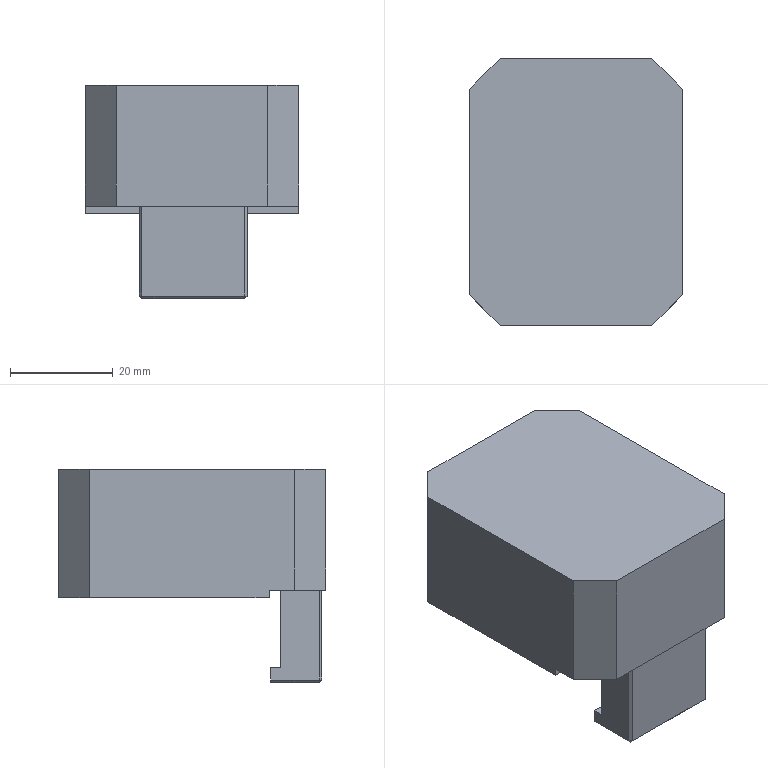Part | SolidWorks | features BaseBody 1 | 1 solid | 26 faces | box 41.5 x 52 x 41.5 mm | volume 54660 mm3 | plane 26
STEP:
#1=CARTESIAN_POINT('',(11.578,-12.01,25.));
#2=VERTEX_POINT('',#1);
#3=CARTESIAN_POINT('',(11.578,27.99,25.));
#4=VERTEX_POINT('',#3);
#5=CARTESIAN_POINT('',(11.578,7.99,25.));
#6=DIRECTION('',(0.,1.,0.));
#7=VECTOR('',#6,1000.);
#8=LINE('',#5,#7);
#9=EDGE_CURVE('',#2,#4,#8,.T.);
#10=ORIENTED_EDGE('',*,*,#9,.T.);
#11=CARTESIAN_POINT('',(5.578,33.99,25.));
#12=VERTEX_POINT('',#11);
#13=CARTESIAN_POINT('',(11.578,27.99,25.));
#14=DIRECTION('',(-0.7071,0.7071,0.));
#15=VECTOR('',#14,1000.);
#16=LINE('',#13,#15);
#17=EDGE_CURVE('',#4,#12,#16,.T.);
#18=ORIENTED_EDGE('',*,*,#17,.T.);
#19=CARTESIAN_POINT('',(-23.922,33.99,25.));
#20=VERTEX_POINT('',#19);
#21=CARTESIAN_POINT('',(-9.172,33.99,25.));
#22=DIRECTION('',(-1.,0.,0.));
#23=VECTOR('',#22,1000.);
#24=LINE('',#21,#23);
#25=EDGE_CURVE('',#12,#20,#24,.T.);
#26=ORIENTED_EDGE('',*,*,#25,.T.);
#27=CARTESIAN_POINT('',(-29.922,27.99,25.));
#28=VERTEX_POINT('',#27);
#29=CARTESIAN_POINT('',(-23.922,33.99,25.));
#30=DIRECTION('',(-0.7071,-0.7071,0.));
#31=VECTOR('',#30,1000.);
#32=LINE('',#29,#31);
#33=EDGE_CURVE('',#20,#28,#32,.T.);
#34=ORIENTED_EDGE('',*,*,#33,.T.);
#35=CARTESIAN_POINT('',(-29.922,-12.01,25.));
#36=VERTEX_POINT('',#35);
#37=CARTESIAN_POINT('',(-29.922,7.99,25.));
#38=DIRECTION('',(0.,-1.,0.));
#39=VECTOR('',#38,1000.);
#40=LINE('',#37,#39);
#41=EDGE_CURVE('',#28,#36,#40,.T.);
#42=ORIENTED_EDGE('',*,*,#41,.T.);
#43=CARTESIAN_POINT('',(-23.922,-18.01,25.));
#44=VERTEX_POINT('',#43);
#45=CARTESIAN_POINT('',(-29.922,-12.01,25.));
#46=DIRECTION('',(0.7071,-0.7071,0.));
#47=VECTOR('',#46,1000.);
#48=LINE('',#45,#47);
#49=EDGE_CURVE('',#36,#44,#48,.T.);
#50=ORIENTED_EDGE('',*,*,#49,.T.);
#51=CARTESIAN_POINT('',(5.578,-18.01,25.));
#52=VERTEX_POINT('',#51);
#53=CARTESIAN_POINT('',(-9.172,-18.01,25.));
#54=DIRECTION('',(1.,0.,0.));
#55=VECTOR('',#54,1000.);
#56=LINE('',#53,#55);
#57=EDGE_CURVE('',#44,#52,#56,.T.);
#58=ORIENTED_EDGE('',*,*,#57,.T.);
#59=CARTESIAN_POINT('',(5.578,-18.01,25.));
#60=DIRECTION('',(0.7071,0.7071,0.));
#61=VECTOR('',#60,1000.);
#62=LINE('',#59,#61);
#63=EDGE_CURVE('',#52,#2,#62,.T.);
#64=ORIENTED_EDGE('',*,*,#63,.T.);
#65=EDGE_LOOP('',(#10,#18,#26,#34,#42,#50,#58,#64));
#66=FACE_OUTER_BOUND('',#65,.T.);
#67=CARTESIAN_POINT('',(-9.172,7.99,25.));
#68=DIRECTION('',(0.,0.,1.));
#69=DIRECTION('',(1.,0.,0.));
#70=AXIS2_PLACEMENT_3D('',#67,#68,#69);
#71=PLANE('',#70);
#72=ADVANCED_FACE('',(#66),#71,.T.);
#73=CARTESIAN_POINT('',(11.578,27.99,0.));
#74=VERTEX_POINT('',#73);
#75=CARTESIAN_POINT('',(5.578,33.99,0.));
#76=VERTEX_POINT('',#75);
#77=CARTESIAN_POINT('',(5.578,33.99,0.));
#78=DIRECTION('',(-0.7071,0.7071,0.));
#79=VECTOR('',#78,1000.);
#80=LINE('',#77,#79);
#81=EDGE_CURVE('',#74,#76,#80,.T.);
#82=ORIENTED_EDGE('',*,*,#81,.T.);
#83=CARTESIAN_POINT('',(5.578,33.99,0.));
#84=DIRECTION('',(0.,0.,1.));
#85=VECTOR('',#84,1000.);
#86=LINE('',#83,#85);
#87=EDGE_CURVE('',#76,#12,#86,.T.);
#88=ORIENTED_EDGE('',*,*,#87,.T.);
#89=ORIENTED_EDGE('',*,*,#17,.F.);
#90=CARTESIAN_POINT('',(11.578,27.99,0.));
#91=DIRECTION('',(0.,0.,-1.));
#92=VECTOR('',#91,1000.);
#93=LINE('',#90,#92);
#94=EDGE_CURVE('',#4,#74,#93,.T.);
#95=ORIENTED_EDGE('',*,*,#94,.T.);
#96=EDGE_LOOP('',(#82,#88,#89,#95));
#97=FACE_OUTER_BOUND('',#96,.T.);
#98=CARTESIAN_POINT('',(5.578,33.99,0.));
#99=DIRECTION('',(0.7071,0.7071,0.));
#100=DIRECTION('',(-0.7071,0.7071,0.));
#101=AXIS2_PLACEMENT_3D('',#98,#99,#100);
#102=PLANE('',#101);
#103=ADVANCED_FACE('',(#97),#102,.T.);
#104=CARTESIAN_POINT('',(11.578,-12.01,1.5));
#105=VERTEX_POINT('',#104);
#106=CARTESIAN_POINT('',(11.578,-12.01,0.));
#107=DIRECTION('',(0.,0.,-1.));
#108=VECTOR('',#107,1000.);
#109=LINE('',#106,#108);
#110=EDGE_CURVE('',#2,#105,#109,.T.);
#111=ORIENTED_EDGE('',*,*,#110,.T.);
#112=CARTESIAN_POINT('',(11.578,-7.01,1.5));
#113=VERTEX_POINT('',#112);
#114=CARTESIAN_POINT('',(11.578,27.99,1.5));
#115=DIRECTION('',(0.,1.,0.));
#116=VECTOR('',#115,1000.);
#117=LINE('',#114,#116);
#118=EDGE_CURVE('',#105,#113,#117,.T.);
#119=ORIENTED_EDGE('',*,*,#118,.T.);
#120=CARTESIAN_POINT('',(11.578,-7.01,0.));
#121=VERTEX_POINT('',#120);
#122=CARTESIAN_POINT('',(11.578,-7.01,0.));
#123=DIRECTION('',(0.,0.,-1.));
#124=VECTOR('',#123,1000.);
#125=LINE('',#122,#124);
#126=EDGE_CURVE('',#113,#121,#125,.T.);
#127=ORIENTED_EDGE('',*,*,#126,.T.);
#128=CARTESIAN_POINT('',(11.578,27.99,0.));
#129=DIRECTION('',(0.,1.,0.));
#130=VECTOR('',#129,1000.);
#131=LINE('',#128,#130);
#132=EDGE_CURVE('',#121,#74,#131,.T.);
#133=ORIENTED_EDGE('',*,*,#132,.T.);
#134=ORIENTED_EDGE('',*,*,#94,.F.);
#135=ORIENTED_EDGE('',*,*,#9,.F.);
#136=EDGE_LOOP('',(#111,#119,#127,#133,#134,#135));
#137=FACE_OUTER_BOUND('',#136,.T.);
#138=CARTESIAN_POINT('',(11.578,27.99,0.));
#139=DIRECTION('',(1.,0.,0.));
#140=DIRECTION('',(0.,0.,-1.));
#141=AXIS2_PLACEMENT_3D('',#138,#139,#140);
#142=PLANE('',#141);
#143=ADVANCED_FACE('',(#137),#142,.T.);
#144=ORIENTED_EDGE('',*,*,#63,.F.);
#145=CARTESIAN_POINT('',(5.578,-18.01,1.5));
#146=VERTEX_POINT('',#145);
#147=CARTESIAN_POINT('',(5.578,-18.01,0.));
#148=DIRECTION('',(0.,0.,-1.));
#149=VECTOR('',#148,1000.);
#150=LINE('',#147,#149);
#151=EDGE_CURVE('',#52,#146,#150,.T.);
#152=ORIENTED_EDGE('',*,*,#151,.T.);
#153=CARTESIAN_POINT('',(11.578,-12.01,1.5));
#154=DIRECTION('',(0.7071,0.7071,0.));
#155=VECTOR('',#154,1000.);
#156=LINE('',#153,#155);
#157=EDGE_CURVE('',#146,#105,#156,.T.);
#158=ORIENTED_EDGE('',*,*,#157,.T.);
#159=ORIENTED_EDGE('',*,*,#110,.F.);
#160=EDGE_LOOP('',(#144,#152,#158,#159));
#161=FACE_OUTER_BOUND('',#160,.T.);
#162=CARTESIAN_POINT('',(11.578,-12.01,0.));
#163=DIRECTION('',(0.7071,-0.7071,0.));
#164=DIRECTION('',(0.7071,0.7071,0.));
#165=AXIS2_PLACEMENT_3D('',#162,#163,#164);
#166=PLANE('',#165);
#167=ADVANCED_FACE('',(#161),#166,.T.);
#168=ORIENTED_EDGE('',*,*,#57,.F.);
#169=CARTESIAN_POINT('',(-23.922,-18.01,1.5));
#170=VERTEX_POINT('',#169);
#171=CARTESIAN_POINT('',(-23.922,-18.01,0.));
#172=DIRECTION('',(0.,0.,-1.));
#173=VECTOR('',#172,1000.);
#174=LINE('',#171,#173);
#175=EDGE_CURVE('',#44,#170,#174,.T.);
#176=ORIENTED_EDGE('',*,*,#175,.T.);
#177=CARTESIAN_POINT('',(5.578,-18.01,1.5));
#178=DIRECTION('',(1.,0.,0.));
#179=VECTOR('',#178,1000.);
#180=LINE('',#177,#179);
#181=EDGE_CURVE('',#170,#146,#180,.T.);
#182=ORIENTED_EDGE('',*,*,#181,.T.);
#183=ORIENTED_EDGE('',*,*,#151,.F.);
#184=EDGE_LOOP('',(#168,#176,#182,#183));
#185=FACE_OUTER_BOUND('',#184,.T.);
#186=CARTESIAN_POINT('',(5.578,-18.01,0.));
#187=DIRECTION('',(0.,-1.,0.));
#188=DIRECTION('',(0.,0.,-1.));
#189=AXIS2_PLACEMENT_3D('',#186,#187,#188);
#190=PLANE('',#189);
#191=ADVANCED_FACE('',(#185),#190,.T.);
#192=ORIENTED_EDGE('',*,*,#49,.F.);
#193=CARTESIAN_POINT('',(-29.922,-12.01,1.5));
#194=VERTEX_POINT('',#193);
#195=CARTESIAN_POINT('',(-29.922,-12.01,0.));
#196=DIRECTION('',(0.,0.,-1.));
#197=VECTOR('',#196,1000.);
#198=LINE('',#195,#197);
#199=EDGE_CURVE('',#36,#194,#198,.T.);
#200=ORIENTED_EDGE('',*,*,#199,.T.);
#201=CARTESIAN_POINT('',(-23.922,-18.01,1.5));
#202=DIRECTION('',(0.7071,-0.7071,0.));
#203=VECTOR('',#202,1000.);
#204=LINE('',#201,#203);
#205=EDGE_CURVE('',#194,#170,#204,.T.);
#206=ORIENTED_EDGE('',*,*,#205,.T.);
#207=ORIENTED_EDGE('',*,*,#175,.F.);
#208=EDGE_LOOP('',(#192,#200,#206,#207));
#209=FACE_OUTER_BOUND('',#208,.T.);
#210=CARTESIAN_POINT('',(-23.922,-18.01,0.));
#211=DIRECTION('',(-0.7071,-0.7071,0.));
#212=DIRECTION('',(0.7071,-0.7071,0.));
#213=AXIS2_PLACEMENT_3D('',#210,#211,#212);
#214=PLANE('',#213);
#215=ADVANCED_FACE('',(#209),#214,.T.);
#216=CARTESIAN_POINT('',(-29.922,27.99,0.));
#217=VERTEX_POINT('',#216);
#218=CARTESIAN_POINT('',(-29.922,-7.01,0.));
#219=VERTEX_POINT('',#218);
#220=CARTESIAN_POINT('',(-29.922,-12.01,0.));
#221=DIRECTION('',(0.,-1.,0.));
#222=VECTOR('',#221,1000.);
#223=LINE('',#220,#222);
#224=EDGE_CURVE('',#217,#219,#223,.T.);
#225=ORIENTED_EDGE('',*,*,#224,.T.);
#226=CARTESIAN_POINT('',(-29.922,-7.01,1.5));
#227=VERTEX_POINT('',#226);
#228=CARTESIAN_POINT('',(-29.922,-7.01,0.));
#229=DIRECTION('',(0.,0.,1.));
#230=VECTOR('',#229,1000.);
#231=LINE('',#228,#230);
#232=EDGE_CURVE('',#219,#227,#231,.T.);
#233=ORIENTED_EDGE('',*,*,#232,.T.);
#234=CARTESIAN_POINT('',(-29.922,-12.01,1.5));
#235=DIRECTION('',(0.,-1.,0.));
#236=VECTOR('',#235,1000.);
#237=LINE('',#234,#236);
#238=EDGE_CURVE('',#227,#194,#237,.T.);
#239=ORIENTED_EDGE('',*,*,#238,.T.);
#240=ORIENTED_EDGE('',*,*,#199,.F.);
#241=ORIENTED_EDGE('',*,*,#41,.F.);
#242=CARTESIAN_POINT('',(-29.922,27.99,0.));
#243=DIRECTION('',(0.,0.,-1.));
#244=VECTOR('',#243,1000.);
#245=LINE('',#242,#244);
#246=EDGE_CURVE('',#28,#217,#245,.T.);
#247=ORIENTED_EDGE('',*,*,#246,.T.);
#248=EDGE_LOOP('',(#225,#233,#239,#240,#241,#247));
#249=FACE_OUTER_BOUND('',#248,.T.);
#250=CARTESIAN_POINT('',(-29.922,-12.01,0.));
#251=DIRECTION('',(-1.,0.,0.));
#252=DIRECTION('',(0.,0.,1.));
#253=AXIS2_PLACEMENT_3D('',#250,#251,#252);
#254=PLANE('',#253);
#255=ADVANCED_FACE('',(#249),#254,.T.);
#256=CARTESIAN_POINT('',(-23.922,33.99,0.));
#257=VERTEX_POINT('',#256);
#258=CARTESIAN_POINT('',(-29.922,27.99,0.));
#259=DIRECTION('',(-0.7071,-0.7071,0.));
#260=VECTOR('',#259,1000.);
#261=LINE('',#258,#260);
#262=EDGE_CURVE('',#257,#217,#261,.T.);
#263=ORIENTED_EDGE('',*,*,#262,.T.);
#264=ORIENTED_EDGE('',*,*,#246,.F.);
#265=ORIENTED_EDGE('',*,*,#33,.F.);
#266=CARTESIAN_POINT('',(-23.922,33.99,0.));
#267=DIRECTION('',(0.,0.,-1.));
#268=VECTOR('',#267,1000.);
#269=LINE('',#266,#268);
#270=EDGE_CURVE('',#20,#257,#269,.T.);
#271=ORIENTED_EDGE('',*,*,#270,.T.);
#272=EDGE_LOOP('',(#263,#264,#265,#271));
#273=FACE_OUTER_BOUND('',#272,.T.);
#274=CARTESIAN_POINT('',(-29.922,27.99,0.));
#275=DIRECTION('',(-0.7071,0.7071,0.));
#276=DIRECTION('',(-0.7071,-0.7071,0.));
#277=AXIS2_PLACEMENT_3D('',#274,#275,#276);
#278=PLANE('',#277);
#279=ADVANCED_FACE('',(#273),#278,.T.);
#280=CARTESIAN_POINT('',(-23.922,33.99,0.));
#281=DIRECTION('',(-1.,0.,0.));
#282=VECTOR('',#281,1000.);
#283=LINE('',#280,#282);
#284=EDGE_CURVE('',#76,#257,#283,.T.);
#285=ORIENTED_EDGE('',*,*,#284,.T.);
#286=ORIENTED_EDGE('',*,*,#270,.F.);
#287=ORIENTED_EDGE('',*,*,#25,.F.);
#288=ORIENTED_EDGE('',*,*,#87,.F.);
#289=EDGE_LOOP('',(#285,#286,#287,#288));
#290=FACE_OUTER_BOUND('',#289,.T.);
#291=CARTESIAN_POINT('',(-23.922,33.99,0.));
#292=DIRECTION('',(0.,1.,0.));
#293=DIRECTION('',(0.,0.,1.));
#294=AXIS2_PLACEMENT_3D('',#291,#292,#293);
#295=PLANE('',#294);
#296=ADVANCED_FACE('',(#290),#295,.T.);
#297=ORIENTED_EDGE('',*,*,#224,.F.);
#298=ORIENTED_EDGE('',*,*,#262,.F.);
#299=ORIENTED_EDGE('',*,*,#284,.F.);
#300=ORIENTED_EDGE('',*,*,#81,.F.);
#301=ORIENTED_EDGE('',*,*,#132,.F.);
#302=CARTESIAN_POINT('',(-9.172,-7.01,0.));
#303=DIRECTION('',(1.,0.,0.));
#304=VECTOR('',#303,1000.);
#305=LINE('',#302,#304);
#306=EDGE_CURVE('',#219,#121,#305,.T.);
#307=ORIENTED_EDGE('',*,*,#306,.F.);
#308=EDGE_LOOP('',(#297,#298,#299,#300,#301,#307));
#309=FACE_OUTER_BOUND('',#308,.T.);
#310=CARTESIAN_POINT('',(-9.172,7.99,0.));
#311=DIRECTION('',(0.,0.,1.));
#312=DIRECTION('',(1.,0.,0.));
#313=AXIS2_PLACEMENT_3D('',#310,#311,#312);
#314=PLANE('',#313);
#315=ADVANCED_FACE('',(#309),#314,.F.);
#316=CARTESIAN_POINT('',(-18.922,-17.31,1.5));
#317=VERTEX_POINT('',#316);
#318=CARTESIAN_POINT('',(-19.422,-16.81,1.5));
#319=VERTEX_POINT('',#318);
#320=CARTESIAN_POINT('',(-19.172,-17.06,1.5));
#321=DIRECTION('',(-0.7071,0.7071,0.));
#322=VECTOR('',#321,1000.);
#323=LINE('',#320,#322);
#324=EDGE_CURVE('',#317,#319,#323,.T.);
#325=ORIENTED_EDGE('',*,*,#324,.F.);
#326=CARTESIAN_POINT('',(1.078,-17.31,1.5));
#327=VERTEX_POINT('',#326);
#328=CARTESIAN_POINT('',(-9.172,-17.31,1.5));
#329=DIRECTION('',(-1.,0.,0.));
#330=VECTOR('',#329,1000.);
#331=LINE('',#328,#330);
#332=EDGE_CURVE('',#327,#317,#331,.T.);
#333=ORIENTED_EDGE('',*,*,#332,.F.);
#334=CARTESIAN_POINT('',(1.578,-16.81,1.5));
#335=VERTEX_POINT('',#334);
#336=CARTESIAN_POINT('',(1.328,-17.06,1.5));
#337=DIRECTION('',(-0.7071,-0.7071,0.));
#338=VECTOR('',#337,1000.);
#339=LINE('',#336,#338);
#340=EDGE_CURVE('',#335,#327,#339,.T.);
#341=ORIENTED_EDGE('',*,*,#340,.F.);
#342=CARTESIAN_POINT('',(1.578,-9.31,1.5));
#343=VERTEX_POINT('',#342);
#344=CARTESIAN_POINT('',(1.578,-11.963,1.5));
#345=DIRECTION('',(0.,-1.,0.));
#346=VECTOR('',#345,1000.);
#347=LINE('',#344,#346);
#348=EDGE_CURVE('',#343,#335,#347,.T.);
#349=ORIENTED_EDGE('',*,*,#348,.F.);
#350=CARTESIAN_POINT('',(-19.422,-9.31,1.5));
#351=VERTEX_POINT('',#350);
#352=CARTESIAN_POINT('',(-9.172,-9.31,1.5));
#353=DIRECTION('',(1.,0.,0.));
#354=VECTOR('',#353,1000.);
#355=LINE('',#352,#354);
#356=EDGE_CURVE('',#351,#343,#355,.T.);
#357=ORIENTED_EDGE('',*,*,#356,.F.);
#358=CARTESIAN_POINT('',(-19.422,-11.963,1.5));
#359=DIRECTION('',(0.,1.,0.));
#360=VECTOR('',#359,1000.);
#361=LINE('',#358,#360);
#362=EDGE_CURVE('',#319,#351,#361,.T.);
#363=ORIENTED_EDGE('',*,*,#362,.F.);
#364=EDGE_LOOP('',(#325,#333,#341,#349,#357,#363));
#365=FACE_BOUND('',#364,.T.);
#366=ORIENTED_EDGE('',*,*,#205,.F.);
#367=ORIENTED_EDGE('',*,*,#238,.F.);
#368=CARTESIAN_POINT('',(-9.172,-7.01,1.5));
#369=DIRECTION('',(-1.,0.,0.));
#370=VECTOR('',#369,1000.);
#371=LINE('',#368,#370);
#372=EDGE_CURVE('',#113,#227,#371,.T.);
#373=ORIENTED_EDGE('',*,*,#372,.F.);
#374=ORIENTED_EDGE('',*,*,#118,.F.);
#375=ORIENTED_EDGE('',*,*,#157,.F.);
#376=ORIENTED_EDGE('',*,*,#181,.F.);
#377=EDGE_LOOP('',(#366,#367,#373,#374,#375,#376));
#378=FACE_OUTER_BOUND('',#377,.T.);
#379=CARTESIAN_POINT('',(-9.172,-11.963,1.5));
#380=DIRECTION('',(0.,0.,1.));
#381=DIRECTION('',(1.,0.,0.));
#382=AXIS2_PLACEMENT_3D('',#379,#380,#381);
#383=PLANE('',#382);
#384=ADVANCED_FACE('',(#365,#378),#383,.F.);
#385=ORIENTED_EDGE('',*,*,#232,.F.);
#386=ORIENTED_EDGE('',*,*,#306,.T.);
#387=ORIENTED_EDGE('',*,*,#126,.F.);
#388=ORIENTED_EDGE('',*,*,#372,.T.);
#389=EDGE_LOOP('',(#385,#386,#387,#388));
#390=FACE_OUTER_BOUND('',#389,.T.);
#391=CARTESIAN_POINT('',(-29.922,-7.01,0.));
#392=DIRECTION('',(0.,1.,0.));
#393=DIRECTION('',(0.,0.,1.));
#394=AXIS2_PLACEMENT_3D('',#391,#392,#393);
#395=PLANE('',#394);
#396=ADVANCED_FACE('',(#390),#395,.F.);
#397=CARTESIAN_POINT('',(-19.422,-7.31,-13.5));
#398=VERTEX_POINT('',#397);
#399=CARTESIAN_POINT('',(-19.422,-7.31,-16.));
#400=VERTEX_POINT('',#399);
#401=CARTESIAN_POINT('',(-19.422,-7.31,1.5));
#402=DIRECTION('',(0.,0.,-1.));
#403=VECTOR('',#402,1000.);
#404=LINE('',#401,#403);
#405=EDGE_CURVE('',#398,#400,#404,.T.);
#406=ORIENTED_EDGE('',*,*,#405,.T.);
#407=CARTESIAN_POINT('',(-19.422,-16.81,-16.));
#408=VERTEX_POINT('',#407);
#409=CARTESIAN_POINT('',(-19.422,-9.31,-16.));
#410=DIRECTION('',(0.,-1.,0.));
#411=VECTOR('',#410,1000.);
#412=LINE('',#409,#411);
#413=EDGE_CURVE('',#400,#408,#412,.T.);
#414=ORIENTED_EDGE('',*,*,#413,.T.);
#415=CARTESIAN_POINT('',(-19.422,-16.81,1.5));
#416=DIRECTION('',(0.,0.,1.));
#417=VECTOR('',#416,1000.);
#418=LINE('',#415,#417);
#419=EDGE_CURVE('',#408,#319,#418,.T.);
#420=ORIENTED_EDGE('',*,*,#419,.T.);
#421=ORIENTED_EDGE('',*,*,#362,.T.);
#422=CARTESIAN_POINT('',(-19.422,-9.31,-13.5));
#423=VERTEX_POINT('',#422);
#424=CARTESIAN_POINT('',(-19.422,-9.31,1.5));
#425=DIRECTION('',(0.,0.,-1.));
#426=VECTOR('',#425,1000.);
#427=LINE('',#424,#426);
#428=EDGE_CURVE('',#351,#423,#427,.T.);
#429=ORIENTED_EDGE('',*,*,#428,.T.);
#430=CARTESIAN_POINT('',(-19.422,-9.31,-13.5));
#431=DIRECTION('',(0.,1.,0.));
#432=VECTOR('',#431,1000.);
#433=LINE('',#430,#432);
#434=EDGE_CURVE('',#423,#398,#433,.T.);
#435=ORIENTED_EDGE('',*,*,#434,.T.);
#436=EDGE_LOOP('',(#406,#414,#420,#421,#429,#435));
#437=FACE_OUTER_BOUND('',#436,.T.);
#438=CARTESIAN_POINT('',(-19.422,-9.31,1.5));
#439=DIRECTION('',(-1.,0.,0.));
#440=DIRECTION('',(0.,0.,1.));
#441=AXIS2_PLACEMENT_3D('',#438,#439,#440);
#442=PLANE('',#441);
#443=ADVANCED_FACE('',(#437),#442,.T.);
#444=CARTESIAN_POINT('',(1.078,-17.31,-16.));
#445=VERTEX_POINT('',#444);
#446=CARTESIAN_POINT('',(1.078,-17.31,1.5));
#447=DIRECTION('',(0.,0.,1.));
#448=VECTOR('',#447,1000.);
#449=LINE('',#446,#448);
#450=EDGE_CURVE('',#445,#327,#449,.T.);
#451=ORIENTED_EDGE('',*,*,#450,.T.);
#452=ORIENTED_EDGE('',*,*,#332,.T.);
#453=CARTESIAN_POINT('',(-18.922,-17.31,-16.));
#454=VERTEX_POINT('',#453);
#455=CARTESIAN_POINT('',(-18.922,-17.31,1.5));
#456=DIRECTION('',(0.,0.,-1.));
#457=VECTOR('',#456,1000.);
#458=LINE('',#455,#457);
#459=EDGE_CURVE('',#317,#454,#458,.T.);
#460=ORIENTED_EDGE('',*,*,#459,.T.);
#461=CARTESIAN_POINT('',(-19.422,-17.31,-16.));
#462=DIRECTION('',(1.,0.,0.));
#463=VECTOR('',#462,1000.);
#464=LINE('',#461,#463);
#465=EDGE_CURVE('',#454,#445,#464,.T.);
#466=ORIENTED_EDGE('',*,*,#465,.T.);
#467=EDGE_LOOP('',(#451,#452,#460,#466));
#468=FACE_OUTER_BOUND('',#467,.T.);
#469=CARTESIAN_POINT('',(-19.422,-17.31,1.5));
#470=DIRECTION('',(0.,-1.,0.));
#471=DIRECTION('',(0.,0.,-1.));
#472=AXIS2_PLACEMENT_3D('',#469,#470,#471);
#473=PLANE('',#472);
#474=ADVANCED_FACE('',(#468),#473,.T.);
#475=CARTESIAN_POINT('',(1.578,-9.31,-13.5));
#476=VERTEX_POINT('',#475);
#477=CARTESIAN_POINT('',(1.578,-9.31,1.5));
#478=DIRECTION('',(0.,0.,1.));
#479=VECTOR('',#478,1000.);
#480=LINE('',#477,#479);
#481=EDGE_CURVE('',#476,#343,#480,.T.);
#482=ORIENTED_EDGE('',*,*,#481,.T.);
#483=ORIENTED_EDGE('',*,*,#348,.T.);
#484=CARTESIAN_POINT('',(1.578,-16.81,-16.));
#485=VERTEX_POINT('',#484);
#486=CARTESIAN_POINT('',(1.578,-16.81,1.5));
#487=DIRECTION('',(0.,0.,-1.));
#488=VECTOR('',#487,1000.);
#489=LINE('',#486,#488);
#490=EDGE_CURVE('',#335,#485,#489,.T.);
#491=ORIENTED_EDGE('',*,*,#490,.T.);
#492=CARTESIAN_POINT('',(1.578,-7.31,-16.));
#493=VERTEX_POINT('',#492);
#494=CARTESIAN_POINT('',(1.578,-17.31,-16.));
#495=DIRECTION('',(0.,1.,0.));
#496=VECTOR('',#495,1000.);
#497=LINE('',#494,#496);
#498=EDGE_CURVE('',#485,#493,#497,.T.);
#499=ORIENTED_EDGE('',*,*,#498,.T.);
#500=CARTESIAN_POINT('',(1.578,-7.31,-13.5));
#501=VERTEX_POINT('',#500);
#502=CARTESIAN_POINT('',(1.578,-7.31,1.5));
#503=DIRECTION('',(0.,0.,1.));
#504=VECTOR('',#503,1000.);
#505=LINE('',#502,#504);
#506=EDGE_CURVE('',#493,#501,#505,.T.);
#507=ORIENTED_EDGE('',*,*,#506,.T.);
#508=CARTESIAN_POINT('',(1.578,-17.31,-13.5));
#509=DIRECTION('',(0.,-1.,0.));
#510=VECTOR('',#509,1000.);
#511=LINE('',#508,#510);
#512=EDGE_CURVE('',#501,#476,#511,.T.);
#513=ORIENTED_EDGE('',*,*,#512,.T.);
#514=EDGE_LOOP('',(#482,#483,#491,#499,#507,#513));
#515=FACE_OUTER_BOUND('',#514,.T.);
#516=CARTESIAN_POINT('',(1.578,-17.31,1.5));
#517=DIRECTION('',(1.,0.,0.));
#518=DIRECTION('',(0.,0.,-1.));
#519=AXIS2_PLACEMENT_3D('',#516,#517,#518);
#520=PLANE('',#519);
#521=ADVANCED_FACE('',(#515),#520,.T.);
#522=ORIENTED_EDGE('',*,*,#356,.T.);
#523=ORIENTED_EDGE('',*,*,#481,.F.);
#524=CARTESIAN_POINT('',(1.578,-9.31,-13.5));
#525=DIRECTION('',(-1.,0.,0.));
#526=VECTOR('',#525,1000.);
#527=LINE('',#524,#526);
#528=EDGE_CURVE('',#476,#423,#527,.T.);
#529=ORIENTED_EDGE('',*,*,#528,.T.);
#530=ORIENTED_EDGE('',*,*,#428,.F.);
#531=EDGE_LOOP('',(#522,#523,#529,#530));
#532=FACE_OUTER_BOUND('',#531,.T.);
#533=CARTESIAN_POINT('',(1.578,-9.31,1.5));
#534=DIRECTION('',(0.,1.,0.));
#535=DIRECTION('',(0.,0.,1.));
#536=AXIS2_PLACEMENT_3D('',#533,#534,#535);
#537=PLANE('',#536);
#538=ADVANCED_FACE('',(#532),#537,.T.);
#539=ORIENTED_EDGE('',*,*,#413,.F.);
#540=CARTESIAN_POINT('',(-18.922,-7.31,-16.5));
#541=VERTEX_POINT('',#540);
#542=CARTESIAN_POINT('',(-19.172,-7.31,-16.25));
#543=DIRECTION('',(0.7071,0.,-0.7071));
#544=VECTOR('',#543,1000.);
#545=LINE('',#542,#544);
#546=EDGE_CURVE('',#400,#541,#545,.T.);
#547=ORIENTED_EDGE('',*,*,#546,.T.);
#548=CARTESIAN_POINT('',(-18.922,-16.81,-16.5));
#549=VERTEX_POINT('',#548);
#550=CARTESIAN_POINT('',(-18.922,-11.31,-16.5));
#551=DIRECTION('',(0.,-1.,0.));
#552=VECTOR('',#551,1000.);
#553=LINE('',#550,#552);
#554=EDGE_CURVE('',#541,#549,#553,.T.);
#555=ORIENTED_EDGE('',*,*,#554,.T.);
#556=CARTESIAN_POINT('',(-19.172,-16.81,-16.25));
#557=DIRECTION('',(-0.7071,0.,0.7071));
#558=VECTOR('',#557,1000.);
#559=LINE('',#556,#558);
#560=EDGE_CURVE('',#549,#408,#559,.T.);
#561=ORIENTED_EDGE('',*,*,#560,.T.);
#562=EDGE_LOOP('',(#539,#547,#555,#561));
#563=FACE_OUTER_BOUND('',#562,.T.);
#564=CARTESIAN_POINT('',(-19.172,-11.31,-16.25));
#565=DIRECTION('',(-0.7071,0.,-0.7071));
#566=DIRECTION('',(-0.7071,0.,0.7071));
#567=AXIS2_PLACEMENT_3D('',#564,#565,#566);
#568=PLANE('',#567);
#569=ADVANCED_FACE('',(#563),#568,.T.);
#570=ORIENTED_EDGE('',*,*,#506,.F.);
#571=CARTESIAN_POINT('',(1.078,-7.31,-16.5));
#572=VERTEX_POINT('',#571);
#573=CARTESIAN_POINT('',(1.578,-7.31,-16.));
#574=DIRECTION('',(-0.7071,0.,-0.7071));
#575=VECTOR('',#574,1000.);
#576=LINE('',#573,#575);
#577=EDGE_CURVE('',#493,#572,#576,.T.);
#578=ORIENTED_EDGE('',*,*,#577,.T.);
#579=CARTESIAN_POINT('',(-8.922,-7.31,-16.5));
#580=DIRECTION('',(-1.,0.,0.));
#581=VECTOR('',#580,1000.);
#582=LINE('',#579,#581);
#583=EDGE_CURVE('',#572,#541,#582,.T.);
#584=ORIENTED_EDGE('',*,*,#583,.T.);
#585=ORIENTED_EDGE('',*,*,#546,.F.);
#586=ORIENTED_EDGE('',*,*,#405,.F.);
#587=CARTESIAN_POINT('',(-8.922,-7.31,-13.5));
#588=DIRECTION('',(1.,0.,0.));
#589=VECTOR('',#588,1000.);
#590=LINE('',#587,#589);
#591=EDGE_CURVE('',#398,#501,#590,.T.);
#592=ORIENTED_EDGE('',*,*,#591,.T.);
#593=EDGE_LOOP('',(#570,#578,#584,#585,#586,#592));
#594=FACE_OUTER_BOUND('',#593,.T.);
#595=CARTESIAN_POINT('',(-8.922,-7.31,-14.979));
#596=DIRECTION('',(0.,1.,0.));
#597=DIRECTION('',(0.,0.,1.));
#598=AXIS2_PLACEMENT_3D('',#595,#596,#597);
#599=PLANE('',#598);
#600=ADVANCED_FACE('',(#594),#599,.T.);
#601=ORIENTED_EDGE('',*,*,#528,.F.);
#602=ORIENTED_EDGE('',*,*,#512,.F.);
#603=ORIENTED_EDGE('',*,*,#591,.F.);
#604=ORIENTED_EDGE('',*,*,#434,.F.);
#605=EDGE_LOOP('',(#601,#602,#603,#604));
#606=FACE_OUTER_BOUND('',#605,.T.);
#607=CARTESIAN_POINT('',(1.578,-9.31,-13.5));
#608=DIRECTION('',(0.,0.,1.));
#609=DIRECTION('',(1.,0.,0.));
#610=AXIS2_PLACEMENT_3D('',#607,#608,#609);
#611=PLANE('',#610);
#612=ADVANCED_FACE('',(#606),#611,.T.);
#613=CARTESIAN_POINT('',(-19.172,-17.06,-16.));
#614=DIRECTION('',(0.7071,-0.7071,0.));
#615=VECTOR('',#614,1000.);
#616=LINE('',#613,#615);
#617=EDGE_CURVE('',#408,#454,#616,.T.);
#618=ORIENTED_EDGE('',*,*,#617,.T.);
#619=ORIENTED_EDGE('',*,*,#459,.F.);
#620=ORIENTED_EDGE('',*,*,#324,.T.);
#621=ORIENTED_EDGE('',*,*,#419,.F.);
#622=EDGE_LOOP('',(#618,#619,#620,#621));
#623=FACE_OUTER_BOUND('',#622,.T.);
#624=CARTESIAN_POINT('',(-19.172,-17.06,1.5));
#625=DIRECTION('',(-0.7071,-0.7071,0.));
#626=DIRECTION('',(0.7071,-0.7071,0.));
#627=AXIS2_PLACEMENT_3D('',#624,#625,#626);
#628=PLANE('',#627);
#629=ADVANCED_FACE('',(#623),#628,.T.);
#630=CARTESIAN_POINT('',(1.328,-17.06,-16.));
#631=DIRECTION('',(0.7071,0.7071,0.));
#632=VECTOR('',#631,1000.);
#633=LINE('',#630,#632);
#634=EDGE_CURVE('',#445,#485,#633,.T.);
#635=ORIENTED_EDGE('',*,*,#634,.T.);
#636=ORIENTED_EDGE('',*,*,#490,.F.);
#637=ORIENTED_EDGE('',*,*,#340,.T.);
#638=ORIENTED_EDGE('',*,*,#450,.F.);
#639=EDGE_LOOP('',(#635,#636,#637,#638));
#640=FACE_OUTER_BOUND('',#639,.T.);
#641=CARTESIAN_POINT('',(1.328,-17.06,1.5));
#642=DIRECTION('',(0.7071,-0.7071,0.));
#643=DIRECTION('',(0.7071,0.7071,0.));
#644=AXIS2_PLACEMENT_3D('',#641,#642,#643);
#645=PLANE('',#644);
#646=ADVANCED_FACE('',(#640),#645,.T.);
#647=CARTESIAN_POINT('',(-18.922,-17.06,-16.25));
#648=DIRECTION('',(0.,0.7071,-0.7071));
#649=VECTOR('',#648,1000.);
#650=LINE('',#647,#649);
#651=EDGE_CURVE('',#454,#549,#650,.T.);
#652=ORIENTED_EDGE('',*,*,#651,.T.);
#653=CARTESIAN_POINT('',(1.078,-16.81,-16.5));
#654=VERTEX_POINT('',#653);
#655=CARTESIAN_POINT('',(-14.172,-16.81,-16.5));
#656=DIRECTION('',(1.,0.,0.));
#657=VECTOR('',#656,1000.);
#658=LINE('',#655,#657);
#659=EDGE_CURVE('',#549,#654,#658,.T.);
#660=ORIENTED_EDGE('',*,*,#659,.T.);
#661=CARTESIAN_POINT('',(1.078,-17.06,-16.25));
#662=DIRECTION('',(0.,-0.7071,0.7071));
#663=VECTOR('',#662,1000.);
#664=LINE('',#661,#663);
#665=EDGE_CURVE('',#654,#445,#664,.T.);
#666=ORIENTED_EDGE('',*,*,#665,.T.);
#667=ORIENTED_EDGE('',*,*,#465,.F.);
#668=EDGE_LOOP('',(#652,#660,#666,#667));
#669=FACE_OUTER_BOUND('',#668,.T.);
#670=CARTESIAN_POINT('',(-14.172,-17.06,-16.25));
#671=DIRECTION('',(0.,-0.7071,-0.7071));
#672=DIRECTION('',(0.,0.7071,-0.7071));
#673=AXIS2_PLACEMENT_3D('',#670,#671,#672);
#674=PLANE('',#673);
#675=ADVANCED_FACE('',(#669),#674,.T.);
#676=CARTESIAN_POINT('',(1.078,-15.31,-16.5));
#677=DIRECTION('',(0.,1.,0.));
#678=VECTOR('',#677,1000.);
#679=LINE('',#676,#678);
#680=EDGE_CURVE('',#654,#572,#679,.T.);
#681=ORIENTED_EDGE('',*,*,#680,.T.);
#682=ORIENTED_EDGE('',*,*,#577,.F.);
#683=ORIENTED_EDGE('',*,*,#498,.F.);
#684=CARTESIAN_POINT('',(1.328,-16.81,-16.25));
#685=DIRECTION('',(-0.7071,0.,-0.7071));
#686=VECTOR('',#685,1000.);
#687=LINE('',#684,#686);
#688=EDGE_CURVE('',#485,#654,#687,.T.);
#689=ORIENTED_EDGE('',*,*,#688,.T.);
#690=EDGE_LOOP('',(#681,#682,#683,#689));
#691=FACE_OUTER_BOUND('',#690,.T.);
#692=CARTESIAN_POINT('',(1.328,-15.31,-16.25));
#693=DIRECTION('',(0.7071,0.,-0.7071));
#694=DIRECTION('',(-0.7071,0.,-0.7071));
#695=AXIS2_PLACEMENT_3D('',#692,#693,#694);
#696=PLANE('',#695);
#697=ADVANCED_FACE('',(#691),#696,.T.);
#698=ORIENTED_EDGE('',*,*,#651,.F.);
#699=ORIENTED_EDGE('',*,*,#617,.F.);
#700=ORIENTED_EDGE('',*,*,#560,.F.);
#701=EDGE_LOOP('',(#698,#699,#700));
#702=FACE_OUTER_BOUND('',#701,.T.);
#703=CARTESIAN_POINT('',(-19.172,-17.06,-16.));
#704=DIRECTION('',(-0.5774,-0.5774,-0.5774));
#705=DIRECTION('',(0.,0.7071,-0.7071));
#706=AXIS2_PLACEMENT_3D('',#703,#704,#705);
#707=PLANE('',#706);
#708=ADVANCED_FACE('',(#702),#707,.T.);
#709=ORIENTED_EDGE('',*,*,#583,.F.);
#710=ORIENTED_EDGE('',*,*,#680,.F.);
#711=ORIENTED_EDGE('',*,*,#659,.F.);
#712=ORIENTED_EDGE('',*,*,#554,.F.);
#713=EDGE_LOOP('',(#709,#710,#711,#712));
#714=FACE_OUTER_BOUND('',#713,.T.);
#715=CARTESIAN_POINT('',(-8.922,-13.31,-16.5));
#716=DIRECTION('',(0.,0.,1.));
#717=DIRECTION('',(1.,0.,0.));
#718=AXIS2_PLACEMENT_3D('',#715,#716,#717);
#719=PLANE('',#718);
#720=ADVANCED_FACE('',(#714),#719,.F.);
#721=ORIENTED_EDGE('',*,*,#688,.F.);
#722=ORIENTED_EDGE('',*,*,#634,.F.);
#723=ORIENTED_EDGE('',*,*,#665,.F.);
#724=EDGE_LOOP('',(#721,#722,#723));
#725=FACE_OUTER_BOUND('',#724,.T.);
#726=CARTESIAN_POINT('',(1.328,-17.06,-16.));
#727=DIRECTION('',(0.5774,-0.5774,-0.5774));
#728=DIRECTION('',(-0.7071,0.,-0.7071));
#729=AXIS2_PLACEMENT_3D('',#726,#727,#728);
#730=PLANE('',#729);
#731=ADVANCED_FACE('',(#725),#730,.T.);
#732=CLOSED_SHELL('',(#72,#103,#143,#167,#191,#215,#255,#279,#296,#315,#384,#396,#443,#474,#521,#538,#569,#600,#612,#629,#646,#675,#697,#708,#720,#731));
#733=MANIFOLD_SOLID_BREP('',#732);
#734=CARTESIAN_POINT('',(0.,0.,0.));
#735=DIRECTION('',(0.,0.,1.));
#736=DIRECTION('',(1.,0.,0.));
#737=AXIS2_PLACEMENT_3D('',#734,#735,#736);
#738=(LENGTH_UNIT()NAMED_UNIT(*)SI_UNIT(.MILLI.,.METRE.));
#739=UNCERTAINTY_MEASURE_WITH_UNIT(LENGTH_MEASURE(0.00001),#738,'','');
#740=(NAMED_UNIT(*)PLANE_ANGLE_UNIT()SI_UNIT($,.RADIAN.));
#741=(NAMED_UNIT(*)SI_UNIT($,.STERADIAN.)SOLID_ANGLE_UNIT());
#742=(GEOMETRIC_REPRESENTATION_CONTEXT(3)GLOBAL_UNCERTAINTY_ASSIGNED_CONTEXT((#739))GLOBAL_UNIT_ASSIGNED_CONTEXT((#738,#740,#741))REPRESENTATION_CONTEXT('',''));
#743=ADVANCED_BREP_SHAPE_REPRESENTATION('',(#733,#737),#742);